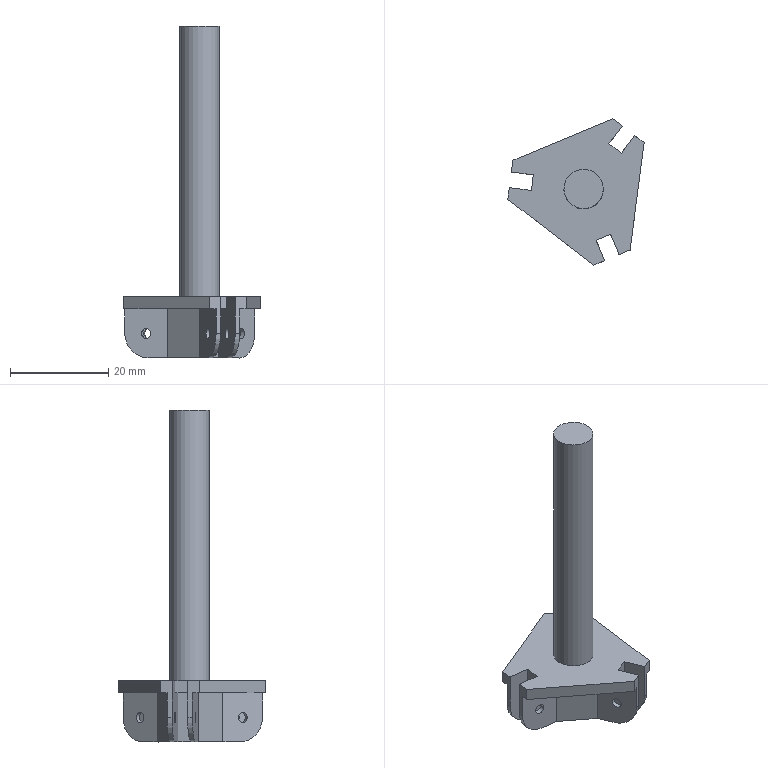Part | NX | features DATUM_CSYS 6, EXTRUDE 5, SKETCH 5, CPROJ 2, EXTRACT_BODY 2, UNITE 2, BLEND 1, BREP 1, DATUM_PLANE 1, Delete Body 1, Pattern Geometry 1 | 1 solid | 52 faces | box 27.712 x 29.745 x 67.5 mm | volume 4749 mm3 | plane 39 | cylinder 13 | commonest cylinder face diameters 2 x6 10 x6 8 x1